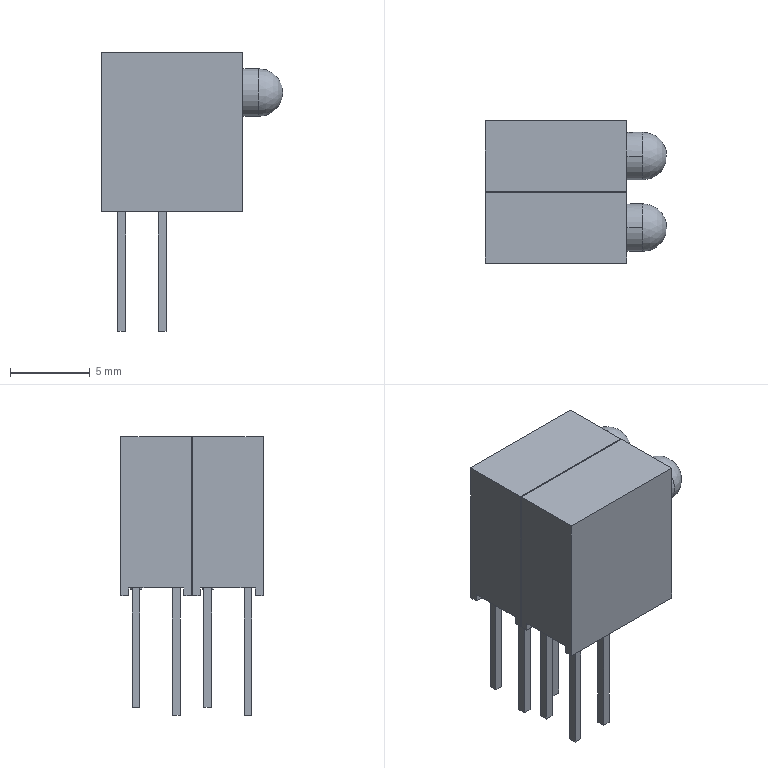Part | SolidWorks | features BaseBody 2 | 2 solids | 78 faces | box 11.4 x 8.95 x 17.5 mm | volume 805.198 mm3 | plane 68 | cylinder 8 | sphere 2 | commonest cylinder face diameters 0.707 x4 3 x4